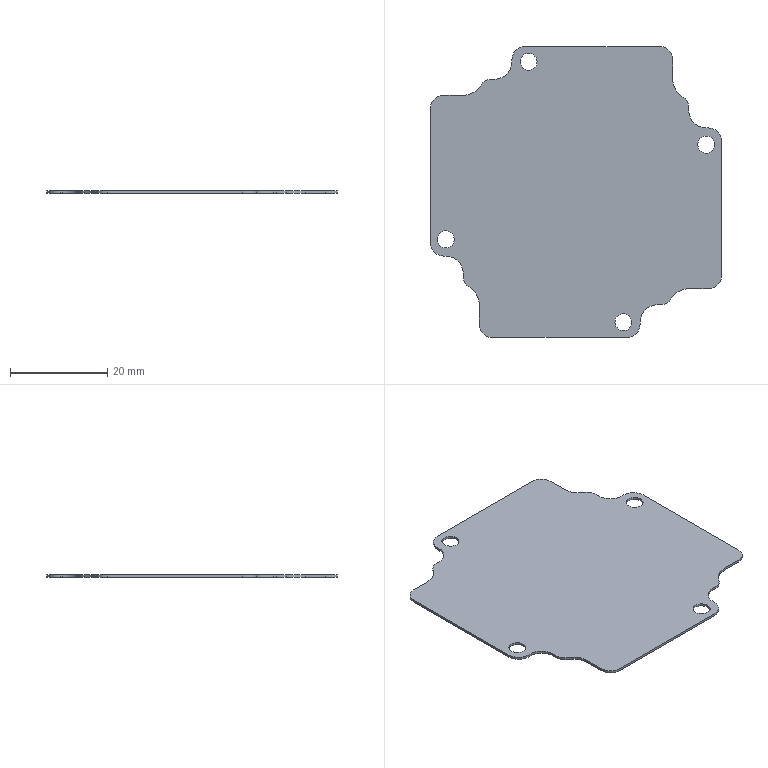Part | STEP file | 1 solid | 42 faces | box 59.8 x 59.8 x 0.5 mm | volume 1478 mm3 | cylinder 24 | plane 18 | commonest cylinder face diameters 5 x8 3.5 x4 5.6 x4 7 x4 9 x4